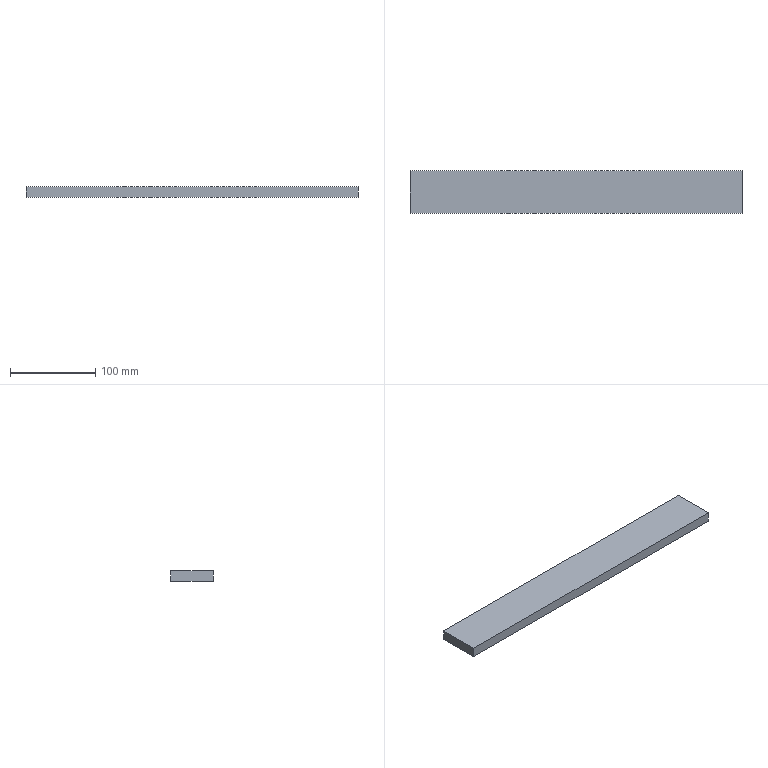Part | NX | features 0008 2 | 1 solid | 6 faces | box 390 x 50 x 12 mm | volume 234000 mm3 | plane 6
STEP:
#1=CARTESIAN_POINT('',(-195.,50.,-12.));
#2=VERTEX_POINT('',#1);
#3=CARTESIAN_POINT('',(-195.,50.,0.));
#4=VERTEX_POINT('',#3);
#5=CARTESIAN_POINT('',(-195.,50.,-12.));
#6=DIRECTION('',(0.,0.,1.));
#7=VECTOR('',#6,1000.);
#8=LINE('',#5,#7);
#9=EDGE_CURVE('',#2,#4,#8,.T.);
#10=ORIENTED_EDGE('',*,*,#9,.T.);
#11=CARTESIAN_POINT('',(195.,50.,0.));
#12=VERTEX_POINT('',#11);
#13=CARTESIAN_POINT('',(-195.,50.,0.));
#14=DIRECTION('',(1.,0.,0.));
#15=VECTOR('',#14,1000.);
#16=LINE('',#13,#15);
#17=EDGE_CURVE('',#4,#12,#16,.T.);
#18=ORIENTED_EDGE('',*,*,#17,.T.);
#19=CARTESIAN_POINT('',(195.,50.,-12.));
#20=VERTEX_POINT('',#19);
#21=CARTESIAN_POINT('',(195.,50.,-12.));
#22=DIRECTION('',(0.,0.,1.));
#23=VECTOR('',#22,1000.);
#24=LINE('',#21,#23);
#25=EDGE_CURVE('',#20,#12,#24,.T.);
#26=ORIENTED_EDGE('',*,*,#25,.F.);
#27=CARTESIAN_POINT('',(-195.,50.,-12.));
#28=DIRECTION('',(1.,0.,0.));
#29=VECTOR('',#28,1000.);
#30=LINE('',#27,#29);
#31=EDGE_CURVE('',#2,#20,#30,.T.);
#32=ORIENTED_EDGE('',*,*,#31,.F.);
#33=EDGE_LOOP('',(#10,#18,#26,#32));
#34=FACE_BOUND('',#33,.T.);
#35=CARTESIAN_POINT('',(195.,50.,0.));
#36=DIRECTION('',(0.,-1.,0.));
#37=DIRECTION('',(0.,0.,1.));
#38=AXIS2_PLACEMENT_3D('',#35,#36,#37);
#39=PLANE('',#38);
#40=ADVANCED_FACE('',(#34),#39,.F.);
#41=CARTESIAN_POINT('',(-195.,0.,-12.));
#42=VERTEX_POINT('',#41);
#43=CARTESIAN_POINT('',(-195.,0.,0.));
#44=VERTEX_POINT('',#43);
#45=CARTESIAN_POINT('',(-195.,0.,-12.));
#46=DIRECTION('',(0.,0.,1.));
#47=VECTOR('',#46,1000.);
#48=LINE('',#45,#47);
#49=EDGE_CURVE('',#42,#44,#48,.T.);
#50=ORIENTED_EDGE('',*,*,#49,.T.);
#51=CARTESIAN_POINT('',(-195.,0.,0.));
#52=DIRECTION('',(0.,1.,0.));
#53=VECTOR('',#52,1000.);
#54=LINE('',#51,#53);
#55=EDGE_CURVE('',#44,#4,#54,.T.);
#56=ORIENTED_EDGE('',*,*,#55,.T.);
#57=ORIENTED_EDGE('',*,*,#9,.F.);
#58=CARTESIAN_POINT('',(-195.,0.,-12.));
#59=DIRECTION('',(0.,1.,0.));
#60=VECTOR('',#59,1000.);
#61=LINE('',#58,#60);
#62=EDGE_CURVE('',#42,#2,#61,.T.);
#63=ORIENTED_EDGE('',*,*,#62,.F.);
#64=EDGE_LOOP('',(#50,#56,#57,#63));
#65=FACE_BOUND('',#64,.T.);
#66=CARTESIAN_POINT('',(-195.,50.,0.));
#67=DIRECTION('',(1.,0.,0.));
#68=DIRECTION('',(0.,0.,-1.));
#69=AXIS2_PLACEMENT_3D('',#66,#67,#68);
#70=PLANE('',#69);
#71=ADVANCED_FACE('',(#65),#70,.F.);
#72=CARTESIAN_POINT('',(195.,0.,0.));
#73=VERTEX_POINT('',#72);
#74=CARTESIAN_POINT('',(195.,50.,0.));
#75=DIRECTION('',(0.,-1.,0.));
#76=VECTOR('',#75,1000.);
#77=LINE('',#74,#76);
#78=EDGE_CURVE('',#12,#73,#77,.T.);
#79=ORIENTED_EDGE('',*,*,#78,.F.);
#80=ORIENTED_EDGE('',*,*,#17,.F.);
#81=ORIENTED_EDGE('',*,*,#55,.F.);
#82=CARTESIAN_POINT('',(195.,0.,0.));
#83=DIRECTION('',(-1.,0.,0.));
#84=VECTOR('',#83,1000.);
#85=LINE('',#82,#84);
#86=EDGE_CURVE('',#73,#44,#85,.T.);
#87=ORIENTED_EDGE('',*,*,#86,.F.);
#88=EDGE_LOOP('',(#79,#80,#81,#87));
#89=FACE_BOUND('',#88,.T.);
#90=CARTESIAN_POINT('',(0.,25.,0.));
#91=DIRECTION('',(0.,0.,1.));
#92=DIRECTION('',(0.,1.,0.));
#93=AXIS2_PLACEMENT_3D('',#90,#91,#92);
#94=PLANE('',#93);
#95=ADVANCED_FACE('',(#89),#94,.T.);
#96=ORIENTED_EDGE('',*,*,#25,.T.);
#97=ORIENTED_EDGE('',*,*,#78,.T.);
#98=CARTESIAN_POINT('',(195.,0.,-12.));
#99=VERTEX_POINT('',#98);
#100=CARTESIAN_POINT('',(195.,0.,-12.));
#101=DIRECTION('',(0.,0.,1.));
#102=VECTOR('',#101,1000.);
#103=LINE('',#100,#102);
#104=EDGE_CURVE('',#99,#73,#103,.T.);
#105=ORIENTED_EDGE('',*,*,#104,.F.);
#106=CARTESIAN_POINT('',(195.,50.,-12.));
#107=DIRECTION('',(0.,-1.,0.));
#108=VECTOR('',#107,1000.);
#109=LINE('',#106,#108);
#110=EDGE_CURVE('',#20,#99,#109,.T.);
#111=ORIENTED_EDGE('',*,*,#110,.F.);
#112=EDGE_LOOP('',(#96,#97,#105,#111));
#113=FACE_BOUND('',#112,.T.);
#114=CARTESIAN_POINT('',(195.,50.,0.));
#115=DIRECTION('',(-1.,0.,0.));
#116=DIRECTION('',(0.,0.,1.));
#117=AXIS2_PLACEMENT_3D('',#114,#115,#116);
#118=PLANE('',#117);
#119=ADVANCED_FACE('',(#113),#118,.F.);
#120=ORIENTED_EDGE('',*,*,#62,.T.);
#121=ORIENTED_EDGE('',*,*,#31,.T.);
#122=ORIENTED_EDGE('',*,*,#110,.T.);
#123=CARTESIAN_POINT('',(195.,0.,-12.));
#124=DIRECTION('',(-1.,0.,0.));
#125=VECTOR('',#124,1000.);
#126=LINE('',#123,#125);
#127=EDGE_CURVE('',#99,#42,#126,.T.);
#128=ORIENTED_EDGE('',*,*,#127,.T.);
#129=EDGE_LOOP('',(#120,#121,#122,#128));
#130=FACE_BOUND('',#129,.T.);
#131=CARTESIAN_POINT('',(0.,25.,-12.));
#132=DIRECTION('',(0.,0.,1.));
#133=DIRECTION('',(0.,1.,0.));
#134=AXIS2_PLACEMENT_3D('',#131,#132,#133);
#135=PLANE('',#134);
#136=ADVANCED_FACE('',(#130),#135,.F.);
#137=ORIENTED_EDGE('',*,*,#104,.T.);
#138=ORIENTED_EDGE('',*,*,#86,.T.);
#139=ORIENTED_EDGE('',*,*,#49,.F.);
#140=ORIENTED_EDGE('',*,*,#127,.F.);
#141=EDGE_LOOP('',(#137,#138,#139,#140));
#142=FACE_BOUND('',#141,.T.);
#143=CARTESIAN_POINT('',(195.,0.,0.));
#144=DIRECTION('',(0.,1.,0.));
#145=DIRECTION('',(0.,0.,-1.));
#146=AXIS2_PLACEMENT_3D('',#143,#144,#145);
#147=PLANE('',#146);
#148=ADVANCED_FACE('',(#142),#147,.F.);
#149=CLOSED_SHELL('',(#40,#71,#95,#119,#136,#148));
#150=MANIFOLD_SOLID_BREP('',#149);
#151=(LENGTH_UNIT()NAMED_UNIT(*)SI_UNIT(.MILLI.,.METRE.));
#152=UNCERTAINTY_MEASURE_WITH_UNIT(LENGTH_MEASURE(0.00001),#151,'','');
#153=(NAMED_UNIT(*)PLANE_ANGLE_UNIT()SI_UNIT($,.RADIAN.));
#154=(NAMED_UNIT(*)SI_UNIT($,.STERADIAN.)SOLID_ANGLE_UNIT());
#155=(GEOMETRIC_REPRESENTATION_CONTEXT(3)GLOBAL_UNCERTAINTY_ASSIGNED_CONTEXT((#152))GLOBAL_UNIT_ASSIGNED_CONTEXT((#151,#153,#154))REPRESENTATION_CONTEXT('',''));
#156=ADVANCED_BREP_SHAPE_REPRESENTATION('',(#150),#155);